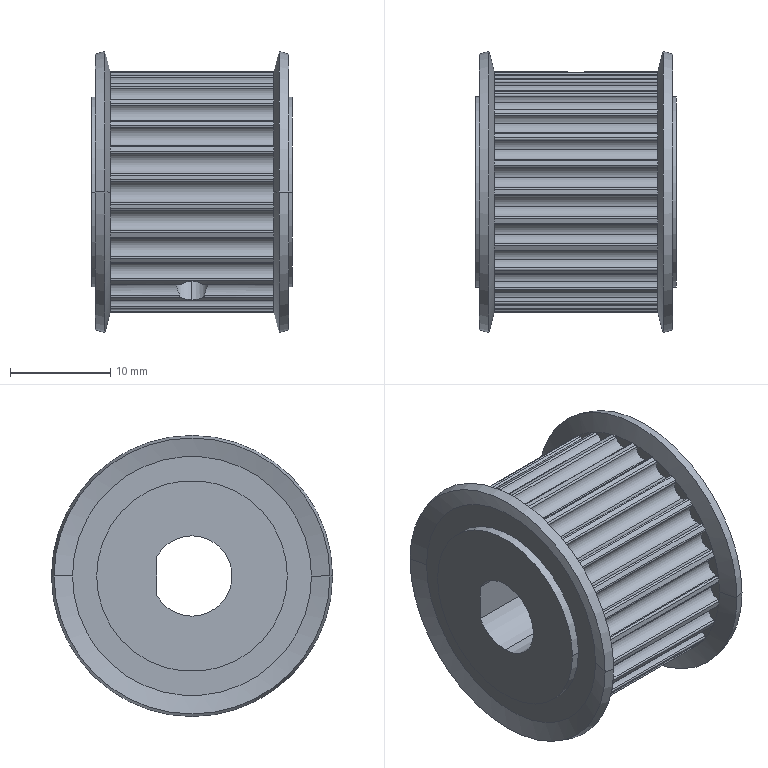Part | NX | features BREP 1 | 1 solid | 218 faces | box 20 x 28 x 28 mm | volume 7218 mm3 | cylinder 148 | plane 58 | cone 12 | commonest cylinder face diameters 0.34 x69 2.06 x40 24.07 x26 3.242 x4 19 x4 8 x3